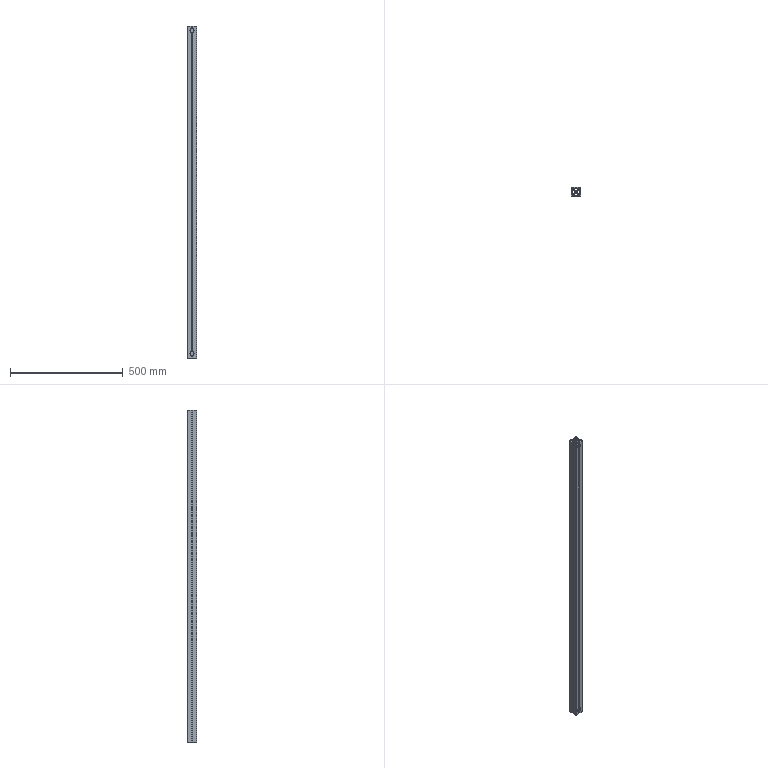Part | STEP file | 09-02 aluminium profile 4040-1470 | 1 solid | 93 faces | box 40 x 40 x 1470 mm | volume 1034180 mm3 | plane 62 | cylinder 31 | commonest cylinder face diameters 19 x9 8 x8 18.5 x8 2 x4 6.8 x2